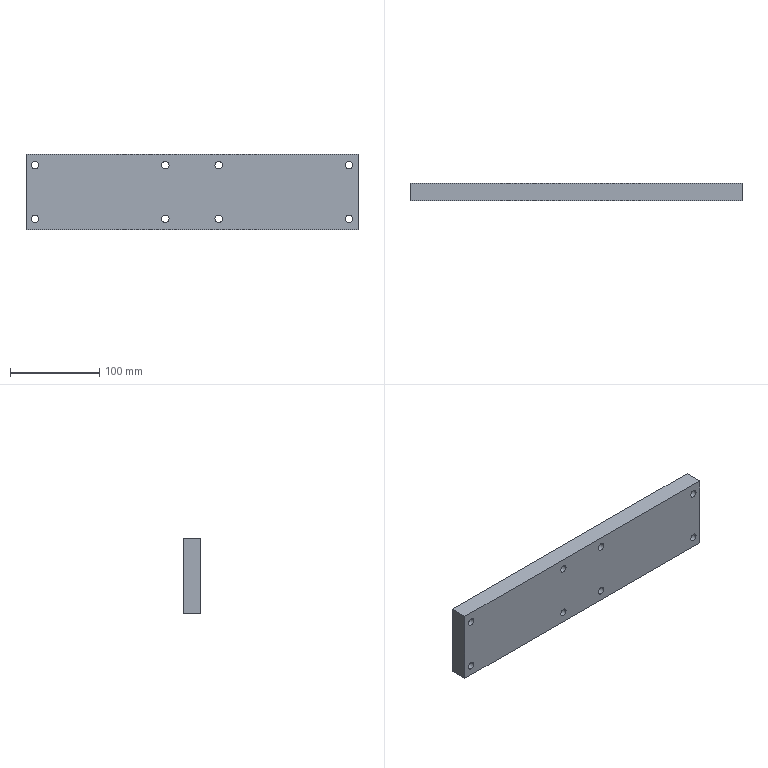Part | NX | features BREP 1 | 1 solid | 46 faces | box 372 x 20 x 85 mm | volume 616323 mm3 | cylinder 32 | plane 14 | commonest cylinder face diameters 8.5 x16 14 x16
STEP:
#1=CARTESIAN_POINT('',(-186.,0.,-42.5));
#2=VERTEX_POINT('',#1);
#3=CARTESIAN_POINT('',(-186.,0.,42.5));
#4=VERTEX_POINT('',#3);
#5=CARTESIAN_POINT('',(-186.,0.,-42.5));
#6=DIRECTION('',(0.,0.,1.));
#7=VECTOR('',#6,1000.);
#8=LINE('',#5,#7);
#9=EDGE_CURVE('',#2,#4,#8,.T.);
#10=ORIENTED_EDGE('',*,*,#9,.F.);
#11=CARTESIAN_POINT('',(186.,0.,-42.5));
#12=VERTEX_POINT('',#11);
#13=CARTESIAN_POINT('',(186.,0.,-42.5));
#14=DIRECTION('',(-1.,0.,0.));
#15=VECTOR('',#14,1000.);
#16=LINE('',#13,#15);
#17=EDGE_CURVE('',#12,#2,#16,.T.);
#18=ORIENTED_EDGE('',*,*,#17,.F.);
#19=CARTESIAN_POINT('',(186.,0.,42.5));
#20=VERTEX_POINT('',#19);
#21=CARTESIAN_POINT('',(186.,0.,42.5));
#22=DIRECTION('',(0.,0.,-1.));
#23=VECTOR('',#22,1000.);
#24=LINE('',#21,#23);
#25=EDGE_CURVE('',#20,#12,#24,.T.);
#26=ORIENTED_EDGE('',*,*,#25,.F.);
#27=CARTESIAN_POINT('',(-186.,0.,42.5));
#28=DIRECTION('',(1.,0.,0.));
#29=VECTOR('',#28,1000.);
#30=LINE('',#27,#29);
#31=EDGE_CURVE('',#4,#20,#30,.T.);
#32=ORIENTED_EDGE('',*,*,#31,.F.);
#33=EDGE_LOOP('',(#10,#18,#26,#32));
#34=FACE_BOUND('',#33,.T.);
#35=CARTESIAN_POINT('',(-34.25,0.,-30.));
#36=VERTEX_POINT('',#35);
#37=CARTESIAN_POINT('',(-25.75,0.,-30.));
#38=VERTEX_POINT('',#37);
#39=CARTESIAN_POINT('',(-30.,0.,-30.));
#40=DIRECTION('',(0.,1.,0.));
#41=DIRECTION('',(-1.,0.,0.));
#42=AXIS2_PLACEMENT_3D('',#39,#40,#41);
#43=CIRCLE('',#42,4.25);
#44=EDGE_CURVE('',#36,#38,#43,.T.);
#45=ORIENTED_EDGE('',*,*,#44,.T.);
#46=CARTESIAN_POINT('',(-30.,0.,-30.));
#47=DIRECTION('',(0.,1.,0.));
#48=DIRECTION('',(1.,0.,0.));
#49=AXIS2_PLACEMENT_3D('',#46,#47,#48);
#50=CIRCLE('',#49,4.25);
#51=EDGE_CURVE('',#38,#36,#50,.T.);
#52=ORIENTED_EDGE('',*,*,#51,.T.);
#53=EDGE_LOOP('',(#45,#52));
#54=FACE_BOUND('',#53,.T.);
#55=CARTESIAN_POINT('',(25.75,0.,-30.));
#56=VERTEX_POINT('',#55);
#57=CARTESIAN_POINT('',(34.25,0.,-30.));
#58=VERTEX_POINT('',#57);
#59=CARTESIAN_POINT('',(30.,0.,-30.));
#60=DIRECTION('',(0.,1.,0.));
#61=DIRECTION('',(-1.,0.,0.));
#62=AXIS2_PLACEMENT_3D('',#59,#60,#61);
#63=CIRCLE('',#62,4.25);
#64=EDGE_CURVE('',#56,#58,#63,.T.);
#65=ORIENTED_EDGE('',*,*,#64,.T.);
#66=CARTESIAN_POINT('',(30.,0.,-30.));
#67=DIRECTION('',(0.,1.,0.));
#68=DIRECTION('',(1.,0.,0.));
#69=AXIS2_PLACEMENT_3D('',#66,#67,#68);
#70=CIRCLE('',#69,4.25);
#71=EDGE_CURVE('',#58,#56,#70,.T.);
#72=ORIENTED_EDGE('',*,*,#71,.T.);
#73=EDGE_LOOP('',(#65,#72));
#74=FACE_BOUND('',#73,.T.);
#75=CARTESIAN_POINT('',(-34.25,0.,30.));
#76=VERTEX_POINT('',#75);
#77=CARTESIAN_POINT('',(-25.75,0.,30.));
#78=VERTEX_POINT('',#77);
#79=CARTESIAN_POINT('',(-30.,0.,30.));
#80=DIRECTION('',(0.,1.,0.));
#81=DIRECTION('',(-1.,0.,0.));
#82=AXIS2_PLACEMENT_3D('',#79,#80,#81);
#83=CIRCLE('',#82,4.25);
#84=EDGE_CURVE('',#76,#78,#83,.T.);
#85=ORIENTED_EDGE('',*,*,#84,.T.);
#86=CARTESIAN_POINT('',(-30.,0.,30.));
#87=DIRECTION('',(0.,1.,0.));
#88=DIRECTION('',(1.,0.,0.));
#89=AXIS2_PLACEMENT_3D('',#86,#87,#88);
#90=CIRCLE('',#89,4.25);
#91=EDGE_CURVE('',#78,#76,#90,.T.);
#92=ORIENTED_EDGE('',*,*,#91,.T.);
#93=EDGE_LOOP('',(#85,#92));
#94=FACE_BOUND('',#93,.T.);
#95=CARTESIAN_POINT('',(25.75,0.,30.));
#96=VERTEX_POINT('',#95);
#97=CARTESIAN_POINT('',(34.25,0.,30.));
#98=VERTEX_POINT('',#97);
#99=CARTESIAN_POINT('',(30.,0.,30.));
#100=DIRECTION('',(0.,1.,0.));
#101=DIRECTION('',(-1.,0.,0.));
#102=AXIS2_PLACEMENT_3D('',#99,#100,#101);
#103=CIRCLE('',#102,4.25);
#104=EDGE_CURVE('',#96,#98,#103,.T.);
#105=ORIENTED_EDGE('',*,*,#104,.T.);
#106=CARTESIAN_POINT('',(30.,0.,30.));
#107=DIRECTION('',(0.,1.,0.));
#108=DIRECTION('',(1.,0.,0.));
#109=AXIS2_PLACEMENT_3D('',#106,#107,#108);
#110=CIRCLE('',#109,4.25);
#111=EDGE_CURVE('',#98,#96,#110,.T.);
#112=ORIENTED_EDGE('',*,*,#111,.T.);
#113=EDGE_LOOP('',(#105,#112));
#114=FACE_BOUND('',#113,.T.);
#115=CARTESIAN_POINT('',(-180.25,0.,-30.));
#116=VERTEX_POINT('',#115);
#117=CARTESIAN_POINT('',(-171.75,0.,-30.));
#118=VERTEX_POINT('',#117);
#119=CARTESIAN_POINT('',(-176.,0.,-30.));
#120=DIRECTION('',(0.,1.,0.));
#121=DIRECTION('',(-1.,0.,0.));
#122=AXIS2_PLACEMENT_3D('',#119,#120,#121);
#123=CIRCLE('',#122,4.25);
#124=EDGE_CURVE('',#116,#118,#123,.T.);
#125=ORIENTED_EDGE('',*,*,#124,.T.);
#126=CARTESIAN_POINT('',(-176.,0.,-30.));
#127=DIRECTION('',(0.,1.,0.));
#128=DIRECTION('',(1.,0.,0.));
#129=AXIS2_PLACEMENT_3D('',#126,#127,#128);
#130=CIRCLE('',#129,4.25);
#131=EDGE_CURVE('',#118,#116,#130,.T.);
#132=ORIENTED_EDGE('',*,*,#131,.T.);
#133=EDGE_LOOP('',(#125,#132));
#134=FACE_BOUND('',#133,.T.);
#135=CARTESIAN_POINT('',(-180.25,0.,30.));
#136=VERTEX_POINT('',#135);
#137=CARTESIAN_POINT('',(-171.75,0.,30.));
#138=VERTEX_POINT('',#137);
#139=CARTESIAN_POINT('',(-176.,0.,30.));
#140=DIRECTION('',(0.,1.,0.));
#141=DIRECTION('',(-1.,0.,0.));
#142=AXIS2_PLACEMENT_3D('',#139,#140,#141);
#143=CIRCLE('',#142,4.25);
#144=EDGE_CURVE('',#136,#138,#143,.T.);
#145=ORIENTED_EDGE('',*,*,#144,.T.);
#146=CARTESIAN_POINT('',(-176.,0.,30.));
#147=DIRECTION('',(0.,1.,0.));
#148=DIRECTION('',(1.,0.,0.));
#149=AXIS2_PLACEMENT_3D('',#146,#147,#148);
#150=CIRCLE('',#149,4.25);
#151=EDGE_CURVE('',#138,#136,#150,.T.);
#152=ORIENTED_EDGE('',*,*,#151,.T.);
#153=EDGE_LOOP('',(#145,#152));
#154=FACE_BOUND('',#153,.T.);
#155=CARTESIAN_POINT('',(171.75,0.,-30.));
#156=VERTEX_POINT('',#155);
#157=CARTESIAN_POINT('',(180.25,0.,-30.));
#158=VERTEX_POINT('',#157);
#159=CARTESIAN_POINT('',(176.,0.,-30.));
#160=DIRECTION('',(0.,1.,0.));
#161=DIRECTION('',(-1.,0.,0.));
#162=AXIS2_PLACEMENT_3D('',#159,#160,#161);
#163=CIRCLE('',#162,4.25);
#164=EDGE_CURVE('',#156,#158,#163,.T.);
#165=ORIENTED_EDGE('',*,*,#164,.T.);
#166=CARTESIAN_POINT('',(176.,0.,-30.));
#167=DIRECTION('',(0.,1.,0.));
#168=DIRECTION('',(1.,0.,0.));
#169=AXIS2_PLACEMENT_3D('',#166,#167,#168);
#170=CIRCLE('',#169,4.25);
#171=EDGE_CURVE('',#158,#156,#170,.T.);
#172=ORIENTED_EDGE('',*,*,#171,.T.);
#173=EDGE_LOOP('',(#165,#172));
#174=FACE_BOUND('',#173,.T.);
#175=CARTESIAN_POINT('',(171.75,0.,30.));
#176=VERTEX_POINT('',#175);
#177=CARTESIAN_POINT('',(180.25,0.,30.));
#178=VERTEX_POINT('',#177);
#179=CARTESIAN_POINT('',(176.,0.,30.));
#180=DIRECTION('',(0.,1.,0.));
#181=DIRECTION('',(-1.,0.,0.));
#182=AXIS2_PLACEMENT_3D('',#179,#180,#181);
#183=CIRCLE('',#182,4.25);
#184=EDGE_CURVE('',#176,#178,#183,.T.);
#185=ORIENTED_EDGE('',*,*,#184,.T.);
#186=CARTESIAN_POINT('',(176.,0.,30.));
#187=DIRECTION('',(0.,1.,0.));
#188=DIRECTION('',(1.,0.,0.));
#189=AXIS2_PLACEMENT_3D('',#186,#187,#188);
#190=CIRCLE('',#189,4.25);
#191=EDGE_CURVE('',#178,#176,#190,.T.);
#192=ORIENTED_EDGE('',*,*,#191,.T.);
#193=EDGE_LOOP('',(#185,#192));
#194=FACE_BOUND('',#193,.T.);
#195=CARTESIAN_POINT('',(0.,0.,0.));
#196=DIRECTION('',(0.,1.,0.));
#197=DIRECTION('',(1.,0.,0.));
#198=AXIS2_PLACEMENT_3D('',#195,#196,#197);
#199=PLANE('',#198);
#200=ADVANCED_FACE('',(#34,#54,#74,#94,#114,#134,#154,#174,#194),#199,.F.);
#201=CARTESIAN_POINT('',(186.,20.,42.5));
#202=VERTEX_POINT('',#201);
#203=CARTESIAN_POINT('',(186.,0.,42.5));
#204=DIRECTION('',(0.,1.,0.));
#205=VECTOR('',#204,1000.);
#206=LINE('',#203,#205);
#207=EDGE_CURVE('',#20,#202,#206,.T.);
#208=ORIENTED_EDGE('',*,*,#207,.T.);
#209=CARTESIAN_POINT('',(-186.,20.,42.5));
#210=VERTEX_POINT('',#209);
#211=CARTESIAN_POINT('',(-186.,20.,42.5));
#212=DIRECTION('',(1.,0.,0.));
#213=VECTOR('',#212,1000.);
#214=LINE('',#211,#213);
#215=EDGE_CURVE('',#210,#202,#214,.T.);
#216=ORIENTED_EDGE('',*,*,#215,.F.);
#217=CARTESIAN_POINT('',(-186.,0.,42.5));
#218=DIRECTION('',(0.,1.,0.));
#219=VECTOR('',#218,1000.);
#220=LINE('',#217,#219);
#221=EDGE_CURVE('',#4,#210,#220,.T.);
#222=ORIENTED_EDGE('',*,*,#221,.F.);
#223=ORIENTED_EDGE('',*,*,#31,.T.);
#224=EDGE_LOOP('',(#208,#216,#222,#223));
#225=FACE_BOUND('',#224,.T.);
#226=CARTESIAN_POINT('',(-186.,0.,42.5));
#227=DIRECTION('',(0.,0.,1.));
#228=DIRECTION('',(1.,0.,0.));
#229=AXIS2_PLACEMENT_3D('',#226,#227,#228);
#230=PLANE('',#229);
#231=ADVANCED_FACE('',(#225),#230,.T.);
#232=ORIENTED_EDGE('',*,*,#221,.T.);
#233=CARTESIAN_POINT('',(-186.,20.,-42.5));
#234=VERTEX_POINT('',#233);
#235=CARTESIAN_POINT('',(-186.,20.,-42.5));
#236=DIRECTION('',(0.,0.,1.));
#237=VECTOR('',#236,1000.);
#238=LINE('',#235,#237);
#239=EDGE_CURVE('',#234,#210,#238,.T.);
#240=ORIENTED_EDGE('',*,*,#239,.F.);
#241=CARTESIAN_POINT('',(-186.,0.,-42.5));
#242=DIRECTION('',(0.,1.,0.));
#243=VECTOR('',#242,1000.);
#244=LINE('',#241,#243);
#245=EDGE_CURVE('',#2,#234,#244,.T.);
#246=ORIENTED_EDGE('',*,*,#245,.F.);
#247=ORIENTED_EDGE('',*,*,#9,.T.);
#248=EDGE_LOOP('',(#232,#240,#246,#247));
#249=FACE_BOUND('',#248,.T.);
#250=CARTESIAN_POINT('',(-186.,0.,-42.5));
#251=DIRECTION('',(-1.,0.,0.));
#252=DIRECTION('',(0.,0.,1.));
#253=AXIS2_PLACEMENT_3D('',#250,#251,#252);
#254=PLANE('',#253);
#255=ADVANCED_FACE('',(#249),#254,.T.);
#256=ORIENTED_EDGE('',*,*,#245,.T.);
#257=CARTESIAN_POINT('',(186.,20.,-42.5));
#258=VERTEX_POINT('',#257);
#259=CARTESIAN_POINT('',(186.,20.,-42.5));
#260=DIRECTION('',(-1.,0.,0.));
#261=VECTOR('',#260,1000.);
#262=LINE('',#259,#261);
#263=EDGE_CURVE('',#258,#234,#262,.T.);
#264=ORIENTED_EDGE('',*,*,#263,.F.);
#265=CARTESIAN_POINT('',(186.,0.,-42.5));
#266=DIRECTION('',(0.,1.,0.));
#267=VECTOR('',#266,1000.);
#268=LINE('',#265,#267);
#269=EDGE_CURVE('',#12,#258,#268,.T.);
#270=ORIENTED_EDGE('',*,*,#269,.F.);
#271=ORIENTED_EDGE('',*,*,#17,.T.);
#272=EDGE_LOOP('',(#256,#264,#270,#271));
#273=FACE_BOUND('',#272,.T.);
#274=CARTESIAN_POINT('',(186.,0.,-42.5));
#275=DIRECTION('',(0.,0.,-1.));
#276=DIRECTION('',(0.,-1.,0.));
#277=AXIS2_PLACEMENT_3D('',#274,#275,#276);
#278=PLANE('',#277);
#279=ADVANCED_FACE('',(#273),#278,.T.);
#280=ORIENTED_EDGE('',*,*,#269,.T.);
#281=CARTESIAN_POINT('',(186.,20.,42.5));
#282=DIRECTION('',(0.,0.,-1.));
#283=VECTOR('',#282,1000.);
#284=LINE('',#281,#283);
#285=EDGE_CURVE('',#202,#258,#284,.T.);
#286=ORIENTED_EDGE('',*,*,#285,.F.);
#287=ORIENTED_EDGE('',*,*,#207,.F.);
#288=ORIENTED_EDGE('',*,*,#25,.T.);
#289=EDGE_LOOP('',(#280,#286,#287,#288));
#290=FACE_BOUND('',#289,.T.);
#291=CARTESIAN_POINT('',(186.,0.,42.5));
#292=DIRECTION('',(1.,0.,0.));
#293=DIRECTION('',(0.,1.,0.));
#294=AXIS2_PLACEMENT_3D('',#291,#292,#293);
#295=PLANE('',#294);
#296=ADVANCED_FACE('',(#290),#295,.T.);
#297=ORIENTED_EDGE('',*,*,#285,.T.);
#298=ORIENTED_EDGE('',*,*,#263,.T.);
#299=ORIENTED_EDGE('',*,*,#239,.T.);
#300=ORIENTED_EDGE('',*,*,#215,.T.);
#301=EDGE_LOOP('',(#297,#298,#299,#300));
#302=FACE_BOUND('',#301,.T.);
#303=CARTESIAN_POINT('',(-37.,20.,-30.));
#304=VERTEX_POINT('',#303);
#305=CARTESIAN_POINT('',(-23.,20.,-30.));
#306=VERTEX_POINT('',#305);
#307=CARTESIAN_POINT('',(-30.,20.,-30.));
#308=DIRECTION('',(0.,1.,0.));
#309=DIRECTION('',(-1.,0.,0.));
#310=AXIS2_PLACEMENT_3D('',#307,#308,#309);
#311=CIRCLE('',#310,7.);
#312=EDGE_CURVE('',#304,#306,#311,.T.);
#313=ORIENTED_EDGE('',*,*,#312,.F.);
#314=CARTESIAN_POINT('',(-30.,20.,-30.));
#315=DIRECTION('',(0.,1.,0.));
#316=DIRECTION('',(1.,0.,0.));
#317=AXIS2_PLACEMENT_3D('',#314,#315,#316);
#318=CIRCLE('',#317,7.);
#319=EDGE_CURVE('',#306,#304,#318,.T.);
#320=ORIENTED_EDGE('',*,*,#319,.F.);
#321=EDGE_LOOP('',(#313,#320));
#322=FACE_BOUND('',#321,.T.);
#323=CARTESIAN_POINT('',(23.,20.,-30.));
#324=VERTEX_POINT('',#323);
#325=CARTESIAN_POINT('',(37.,20.,-30.));
#326=VERTEX_POINT('',#325);
#327=CARTESIAN_POINT('',(30.,20.,-30.));
#328=DIRECTION('',(0.,1.,0.));
#329=DIRECTION('',(-1.,0.,0.));
#330=AXIS2_PLACEMENT_3D('',#327,#328,#329);
#331=CIRCLE('',#330,7.);
#332=EDGE_CURVE('',#324,#326,#331,.T.);
#333=ORIENTED_EDGE('',*,*,#332,.F.);
#334=CARTESIAN_POINT('',(30.,20.,-30.));
#335=DIRECTION('',(0.,1.,0.));
#336=DIRECTION('',(1.,0.,0.));
#337=AXIS2_PLACEMENT_3D('',#334,#335,#336);
#338=CIRCLE('',#337,7.);
#339=EDGE_CURVE('',#326,#324,#338,.T.);
#340=ORIENTED_EDGE('',*,*,#339,.F.);
#341=EDGE_LOOP('',(#333,#340));
#342=FACE_BOUND('',#341,.T.);
#343=CARTESIAN_POINT('',(-37.,20.,30.));
#344=VERTEX_POINT('',#343);
#345=CARTESIAN_POINT('',(-23.,20.,30.));
#346=VERTEX_POINT('',#345);
#347=CARTESIAN_POINT('',(-30.,20.,30.));
#348=DIRECTION('',(0.,1.,0.));
#349=DIRECTION('',(-1.,0.,0.));
#350=AXIS2_PLACEMENT_3D('',#347,#348,#349);
#351=CIRCLE('',#350,7.);
#352=EDGE_CURVE('',#344,#346,#351,.T.);
#353=ORIENTED_EDGE('',*,*,#352,.F.);
#354=CARTESIAN_POINT('',(-30.,20.,30.));
#355=DIRECTION('',(0.,1.,0.));
#356=DIRECTION('',(1.,0.,0.));
#357=AXIS2_PLACEMENT_3D('',#354,#355,#356);
#358=CIRCLE('',#357,7.);
#359=EDGE_CURVE('',#346,#344,#358,.T.);
#360=ORIENTED_EDGE('',*,*,#359,.F.);
#361=EDGE_LOOP('',(#353,#360));
#362=FACE_BOUND('',#361,.T.);
#363=CARTESIAN_POINT('',(23.,20.,30.));
#364=VERTEX_POINT('',#363);
#365=CARTESIAN_POINT('',(37.,20.,30.));
#366=VERTEX_POINT('',#365);
#367=CARTESIAN_POINT('',(30.,20.,30.));
#368=DIRECTION('',(0.,1.,0.));
#369=DIRECTION('',(-1.,0.,0.));
#370=AXIS2_PLACEMENT_3D('',#367,#368,#369);
#371=CIRCLE('',#370,7.);
#372=EDGE_CURVE('',#364,#366,#371,.T.);
#373=ORIENTED_EDGE('',*,*,#372,.F.);
#374=CARTESIAN_POINT('',(30.,20.,30.));
#375=DIRECTION('',(0.,1.,0.));
#376=DIRECTION('',(1.,0.,0.));
#377=AXIS2_PLACEMENT_3D('',#374,#375,#376);
#378=CIRCLE('',#377,7.);
#379=EDGE_CURVE('',#366,#364,#378,.T.);
#380=ORIENTED_EDGE('',*,*,#379,.F.);
#381=EDGE_LOOP('',(#373,#380));
#382=FACE_BOUND('',#381,.T.);
#383=CARTESIAN_POINT('',(-183.,20.,-30.));
#384=VERTEX_POINT('',#383);
#385=CARTESIAN_POINT('',(-169.,20.,-30.));
#386=VERTEX_POINT('',#385);
#387=CARTESIAN_POINT('',(-176.,20.,-30.));
#388=DIRECTION('',(0.,1.,0.));
#389=DIRECTION('',(-1.,0.,0.));
#390=AXIS2_PLACEMENT_3D('',#387,#388,#389);
#391=CIRCLE('',#390,7.);
#392=EDGE_CURVE('',#384,#386,#391,.T.);
#393=ORIENTED_EDGE('',*,*,#392,.F.);
#394=CARTESIAN_POINT('',(-176.,20.,-30.));
#395=DIRECTION('',(0.,1.,0.));
#396=DIRECTION('',(1.,0.,0.));
#397=AXIS2_PLACEMENT_3D('',#394,#395,#396);
#398=CIRCLE('',#397,7.);
#399=EDGE_CURVE('',#386,#384,#398,.T.);
#400=ORIENTED_EDGE('',*,*,#399,.F.);
#401=EDGE_LOOP('',(#393,#400));
#402=FACE_BOUND('',#401,.T.);
#403=CARTESIAN_POINT('',(-183.,20.,30.));
#404=VERTEX_POINT('',#403);
#405=CARTESIAN_POINT('',(-169.,20.,30.));
#406=VERTEX_POINT('',#405);
#407=CARTESIAN_POINT('',(-176.,20.,30.));
#408=DIRECTION('',(0.,1.,0.));
#409=DIRECTION('',(-1.,0.,0.));
#410=AXIS2_PLACEMENT_3D('',#407,#408,#409);
#411=CIRCLE('',#410,7.);
#412=EDGE_CURVE('',#404,#406,#411,.T.);
#413=ORIENTED_EDGE('',*,*,#412,.F.);
#414=CARTESIAN_POINT('',(-176.,20.,30.));
#415=DIRECTION('',(0.,1.,0.));
#416=DIRECTION('',(1.,0.,0.));
#417=AXIS2_PLACEMENT_3D('',#414,#415,#416);
#418=CIRCLE('',#417,7.);
#419=EDGE_CURVE('',#406,#404,#418,.T.);
#420=ORIENTED_EDGE('',*,*,#419,.F.);
#421=EDGE_LOOP('',(#413,#420));
#422=FACE_BOUND('',#421,.T.);
#423=CARTESIAN_POINT('',(169.,20.,-30.));
#424=VERTEX_POINT('',#423);
#425=CARTESIAN_POINT('',(183.,20.,-30.));
#426=VERTEX_POINT('',#425);
#427=CARTESIAN_POINT('',(176.,20.,-30.));
#428=DIRECTION('',(0.,1.,0.));
#429=DIRECTION('',(-1.,0.,0.));
#430=AXIS2_PLACEMENT_3D('',#427,#428,#429);
#431=CIRCLE('',#430,7.);
#432=EDGE_CURVE('',#424,#426,#431,.T.);
#433=ORIENTED_EDGE('',*,*,#432,.F.);
#434=CARTESIAN_POINT('',(176.,20.,-30.));
#435=DIRECTION('',(0.,1.,0.));
#436=DIRECTION('',(1.,0.,0.));
#437=AXIS2_PLACEMENT_3D('',#434,#435,#436);
#438=CIRCLE('',#437,7.);
#439=EDGE_CURVE('',#426,#424,#438,.T.);
#440=ORIENTED_EDGE('',*,*,#439,.F.);
#441=EDGE_LOOP('',(#433,#440));
#442=FACE_BOUND('',#441,.T.);
#443=CARTESIAN_POINT('',(169.,20.,30.));
#444=VERTEX_POINT('',#443);
#445=CARTESIAN_POINT('',(183.,20.,30.));
#446=VERTEX_POINT('',#445);
#447=CARTESIAN_POINT('',(176.,20.,30.));
#448=DIRECTION('',(0.,1.,0.));
#449=DIRECTION('',(-1.,0.,0.));
#450=AXIS2_PLACEMENT_3D('',#447,#448,#449);
#451=CIRCLE('',#450,7.);
#452=EDGE_CURVE('',#444,#446,#451,.T.);
#453=ORIENTED_EDGE('',*,*,#452,.F.);
#454=CARTESIAN_POINT('',(176.,20.,30.));
#455=DIRECTION('',(0.,1.,0.));
#456=DIRECTION('',(1.,0.,0.));
#457=AXIS2_PLACEMENT_3D('',#454,#455,#456);
#458=CIRCLE('',#457,7.);
#459=EDGE_CURVE('',#446,#444,#458,.T.);
#460=ORIENTED_EDGE('',*,*,#459,.F.);
#461=EDGE_LOOP('',(#453,#460));
#462=FACE_BOUND('',#461,.T.);
#463=CARTESIAN_POINT('',(0.,20.,0.));
#464=DIRECTION('',(0.,1.,0.));
#465=DIRECTION('',(1.,0.,0.));
#466=AXIS2_PLACEMENT_3D('',#463,#464,#465);
#467=PLANE('',#466);
#468=ADVANCED_FACE('',(#302,#322,#342,#362,#382,#402,#422,#442,#462),#467,.T.);
#469=CARTESIAN_POINT('',(-37.,11.,-30.));
#470=VERTEX_POINT('',#469);
#471=CARTESIAN_POINT('',(-37.,11.,-30.));
#472=DIRECTION('',(0.,1.,0.));
#473=VECTOR('',#472,1000.);
#474=LINE('',#471,#473);
#475=EDGE_CURVE('',#470,#304,#474,.T.);
#476=ORIENTED_EDGE('',*,*,#475,.F.);
#477=CARTESIAN_POINT('',(-23.,11.,-30.));
#478=VERTEX_POINT('',#477);
#479=CARTESIAN_POINT('',(-30.,11.,-30.));
#480=DIRECTION('',(0.,1.,0.));
#481=DIRECTION('',(1.,0.,0.));
#482=AXIS2_PLACEMENT_3D('',#479,#480,#481);
#483=CIRCLE('',#482,7.);
#484=EDGE_CURVE('',#478,#470,#483,.T.);
#485=ORIENTED_EDGE('',*,*,#484,.F.);
#486=CARTESIAN_POINT('',(-23.,11.,-30.));
#487=DIRECTION('',(0.,1.,0.));
#488=VECTOR('',#487,1000.);
#489=LINE('',#486,#488);
#490=EDGE_CURVE('',#478,#306,#489,.T.);
#491=ORIENTED_EDGE('',*,*,#490,.T.);
#492=ORIENTED_EDGE('',*,*,#319,.T.);
#493=EDGE_LOOP('',(#476,#485,#491,#492));
#494=FACE_BOUND('',#493,.T.);
#495=CARTESIAN_POINT('',(-30.,-73.622,-30.));
#496=DIRECTION('',(0.,1.,0.));
#497=DIRECTION('',(1.,0.,0.));
#498=AXIS2_PLACEMENT_3D('',#495,#496,#497);
#499=CYLINDRICAL_SURFACE('',#498,7.);
#500=ADVANCED_FACE('',(#494),#499,.F.);
#501=ORIENTED_EDGE('',*,*,#490,.F.);
#502=CARTESIAN_POINT('',(-30.,11.,-30.));
#503=DIRECTION('',(0.,-1.,0.));
#504=DIRECTION('',(1.,0.,0.));
#505=AXIS2_PLACEMENT_3D('',#502,#503,#504);
#506=CIRCLE('',#505,7.);
#507=EDGE_CURVE('',#478,#470,#506,.T.);
#508=ORIENTED_EDGE('',*,*,#507,.T.);
#509=ORIENTED_EDGE('',*,*,#475,.T.);
#510=ORIENTED_EDGE('',*,*,#312,.T.);
#511=EDGE_LOOP('',(#501,#508,#509,#510));
#512=FACE_BOUND('',#511,.T.);
#513=CARTESIAN_POINT('',(-30.,-73.622,-30.));
#514=DIRECTION('',(0.,1.,0.));
#515=DIRECTION('',(1.,0.,0.));
#516=AXIS2_PLACEMENT_3D('',#513,#514,#515);
#517=CYLINDRICAL_SURFACE('',#516,7.);
#518=ADVANCED_FACE('',(#512),#517,.F.);
#519=ORIENTED_EDGE('',*,*,#507,.F.);
#520=ORIENTED_EDGE('',*,*,#484,.T.);
#521=EDGE_LOOP('',(#519,#520));
#522=FACE_BOUND('',#521,.T.);
#523=CARTESIAN_POINT('',(-25.75,11.,-30.));
#524=VERTEX_POINT('',#523);
#525=CARTESIAN_POINT('',(-34.25,11.,-30.));
#526=VERTEX_POINT('',#525);
#527=CARTESIAN_POINT('',(-30.,11.,-30.));
#528=DIRECTION('',(0.,1.,0.));
#529=DIRECTION('',(1.,0.,0.));
#530=AXIS2_PLACEMENT_3D('',#527,#528,#529);
#531=CIRCLE('',#530,4.25);
#532=EDGE_CURVE('',#524,#526,#531,.T.);
#533=ORIENTED_EDGE('',*,*,#532,.F.);
#534=CARTESIAN_POINT('',(-30.,11.,-30.));
#535=DIRECTION('',(0.,-1.,0.));
#536=DIRECTION('',(1.,0.,0.));
#537=AXIS2_PLACEMENT_3D('',#534,#535,#536);
#538=CIRCLE('',#537,4.25);
#539=EDGE_CURVE('',#524,#526,#538,.T.);
#540=ORIENTED_EDGE('',*,*,#539,.T.);
#541=EDGE_LOOP('',(#533,#540));
#542=FACE_BOUND('',#541,.T.);
#543=CARTESIAN_POINT('',(-30.,11.,-30.));
#544=DIRECTION('',(0.,1.,0.));
#545=DIRECTION('',(1.,0.,0.));
#546=AXIS2_PLACEMENT_3D('',#543,#544,#545);
#547=PLANE('',#546);
#548=ADVANCED_FACE('',(#522,#542),#547,.T.);
#549=ORIENTED_EDGE('',*,*,#44,.F.);
#550=CARTESIAN_POINT('',(-34.25,0.,-30.));
#551=DIRECTION('',(0.,1.,0.));
#552=VECTOR('',#551,1000.);
#553=LINE('',#550,#552);
#554=EDGE_CURVE('',#526,#36,#553,.F.);
#555=ORIENTED_EDGE('',*,*,#554,.F.);
#556=ORIENTED_EDGE('',*,*,#539,.F.);
#557=CARTESIAN_POINT('',(-25.75,0.,-30.));
#558=DIRECTION('',(0.,1.,0.));
#559=VECTOR('',#558,1000.);
#560=LINE('',#557,#559);
#561=EDGE_CURVE('',#524,#38,#560,.F.);
#562=ORIENTED_EDGE('',*,*,#561,.T.);
#563=EDGE_LOOP('',(#549,#555,#556,#562));
#564=FACE_BOUND('',#563,.T.);
#565=CARTESIAN_POINT('',(-30.,-73.622,-30.));
#566=DIRECTION('',(0.,1.,0.));
#567=DIRECTION('',(1.,0.,0.));
#568=AXIS2_PLACEMENT_3D('',#565,#566,#567);
#569=CYLINDRICAL_SURFACE('',#568,4.25);
#570=ADVANCED_FACE('',(#564),#569,.F.);
#571=ORIENTED_EDGE('',*,*,#532,.T.);
#572=ORIENTED_EDGE('',*,*,#554,.T.);
#573=ORIENTED_EDGE('',*,*,#51,.F.);
#574=ORIENTED_EDGE('',*,*,#561,.F.);
#575=EDGE_LOOP('',(#571,#572,#573,#574));
#576=FACE_BOUND('',#575,.T.);
#577=CARTESIAN_POINT('',(-30.,-73.622,-30.));
#578=DIRECTION('',(0.,1.,0.));
#579=DIRECTION('',(1.,0.,0.));
#580=AXIS2_PLACEMENT_3D('',#577,#578,#579);
#581=CYLINDRICAL_SURFACE('',#580,4.25);
#582=ADVANCED_FACE('',(#576),#581,.F.);
#583=CARTESIAN_POINT('',(23.,11.,-30.));
#584=VERTEX_POINT('',#583);
#585=CARTESIAN_POINT('',(23.,11.,-30.));
#586=DIRECTION('',(0.,1.,0.));
#587=VECTOR('',#586,1000.);
#588=LINE('',#585,#587);
#589=EDGE_CURVE('',#584,#324,#588,.T.);
#590=ORIENTED_EDGE('',*,*,#589,.F.);
#591=CARTESIAN_POINT('',(37.,11.,-30.));
#592=VERTEX_POINT('',#591);
#593=CARTESIAN_POINT('',(30.,11.,-30.));
#594=DIRECTION('',(0.,1.,0.));
#595=DIRECTION('',(1.,0.,0.));
#596=AXIS2_PLACEMENT_3D('',#593,#594,#595);
#597=CIRCLE('',#596,7.);
#598=EDGE_CURVE('',#592,#584,#597,.T.);
#599=ORIENTED_EDGE('',*,*,#598,.F.);
#600=CARTESIAN_POINT('',(37.,11.,-30.));
#601=DIRECTION('',(0.,1.,0.));
#602=VECTOR('',#601,1000.);
#603=LINE('',#600,#602);
#604=EDGE_CURVE('',#592,#326,#603,.T.);
#605=ORIENTED_EDGE('',*,*,#604,.T.);
#606=ORIENTED_EDGE('',*,*,#339,.T.);
#607=EDGE_LOOP('',(#590,#599,#605,#606));
#608=FACE_BOUND('',#607,.T.);
#609=CARTESIAN_POINT('',(30.,-73.622,-30.));
#610=DIRECTION('',(0.,1.,0.));
#611=DIRECTION('',(1.,0.,0.));
#612=AXIS2_PLACEMENT_3D('',#609,#610,#611);
#613=CYLINDRICAL_SURFACE('',#612,7.);
#614=ADVANCED_FACE('',(#608),#613,.F.);
#615=ORIENTED_EDGE('',*,*,#604,.F.);
#616=CARTESIAN_POINT('',(30.,11.,-30.));
#617=DIRECTION('',(0.,-1.,0.));
#618=DIRECTION('',(1.,0.,0.));
#619=AXIS2_PLACEMENT_3D('',#616,#617,#618);
#620=CIRCLE('',#619,7.);
#621=EDGE_CURVE('',#592,#584,#620,.T.);
#622=ORIENTED_EDGE('',*,*,#621,.T.);
#623=ORIENTED_EDGE('',*,*,#589,.T.);
#624=ORIENTED_EDGE('',*,*,#332,.T.);
#625=EDGE_LOOP('',(#615,#622,#623,#624));
#626=FACE_BOUND('',#625,.T.);
#627=CARTESIAN_POINT('',(30.,-73.622,-30.));
#628=DIRECTION('',(0.,1.,0.));
#629=DIRECTION('',(1.,0.,0.));
#630=AXIS2_PLACEMENT_3D('',#627,#628,#629);
#631=CYLINDRICAL_SURFACE('',#630,7.);
#632=ADVANCED_FACE('',(#626),#631,.F.);
#633=ORIENTED_EDGE('',*,*,#621,.F.);
#634=ORIENTED_EDGE('',*,*,#598,.T.);
#635=EDGE_LOOP('',(#633,#634));
#636=FACE_BOUND('',#635,.T.);
#637=CARTESIAN_POINT('',(34.25,11.,-30.));
#638=VERTEX_POINT('',#637);
#639=CARTESIAN_POINT('',(25.75,11.,-30.));
#640=VERTEX_POINT('',#639);
#641=CARTESIAN_POINT('',(30.,11.,-30.));
#642=DIRECTION('',(0.,1.,0.));
#643=DIRECTION('',(1.,0.,0.));
#644=AXIS2_PLACEMENT_3D('',#641,#642,#643);
#645=CIRCLE('',#644,4.25);
#646=EDGE_CURVE('',#638,#640,#645,.T.);
#647=ORIENTED_EDGE('',*,*,#646,.F.);
#648=CARTESIAN_POINT('',(30.,11.,-30.));
#649=DIRECTION('',(0.,-1.,0.));
#650=DIRECTION('',(1.,0.,0.));
#651=AXIS2_PLACEMENT_3D('',#648,#649,#650);
#652=CIRCLE('',#651,4.25);
#653=EDGE_CURVE('',#638,#640,#652,.T.);
#654=ORIENTED_EDGE('',*,*,#653,.T.);
#655=EDGE_LOOP('',(#647,#654));
#656=FACE_BOUND('',#655,.T.);
#657=CARTESIAN_POINT('',(30.,11.,-30.));
#658=DIRECTION('',(0.,1.,0.));
#659=DIRECTION('',(1.,0.,0.));
#660=AXIS2_PLACEMENT_3D('',#657,#658,#659);
#661=PLANE('',#660);
#662=ADVANCED_FACE('',(#636,#656),#661,.T.);
#663=ORIENTED_EDGE('',*,*,#64,.F.);
#664=CARTESIAN_POINT('',(25.75,0.,-30.));
#665=DIRECTION('',(0.,1.,0.));
#666=VECTOR('',#665,1000.);
#667=LINE('',#664,#666);
#668=EDGE_CURVE('',#640,#56,#667,.F.);
#669=ORIENTED_EDGE('',*,*,#668,.F.);
#670=ORIENTED_EDGE('',*,*,#653,.F.);
#671=CARTESIAN_POINT('',(34.25,0.,-30.));
#672=DIRECTION('',(0.,1.,0.));
#673=VECTOR('',#672,1000.);
#674=LINE('',#671,#673);
#675=EDGE_CURVE('',#638,#58,#674,.F.);
#676=ORIENTED_EDGE('',*,*,#675,.T.);
#677=EDGE_LOOP('',(#663,#669,#670,#676));
#678=FACE_BOUND('',#677,.T.);
#679=CARTESIAN_POINT('',(30.,-73.622,-30.));
#680=DIRECTION('',(0.,1.,0.));
#681=DIRECTION('',(1.,0.,0.));
#682=AXIS2_PLACEMENT_3D('',#679,#680,#681);
#683=CYLINDRICAL_SURFACE('',#682,4.25);
#684=ADVANCED_FACE('',(#678),#683,.F.);
#685=ORIENTED_EDGE('',*,*,#646,.T.);
#686=ORIENTED_EDGE('',*,*,#668,.T.);
#687=ORIENTED_EDGE('',*,*,#71,.F.);
#688=ORIENTED_EDGE('',*,*,#675,.F.);
#689=EDGE_LOOP('',(#685,#686,#687,#688));
#690=FACE_BOUND('',#689,.T.);
#691=CARTESIAN_POINT('',(30.,-73.622,-30.));
#692=DIRECTION('',(0.,1.,0.));
#693=DIRECTION('',(1.,0.,0.));
#694=AXIS2_PLACEMENT_3D('',#691,#692,#693);
#695=CYLINDRICAL_SURFACE('',#694,4.25);
#696=ADVANCED_FACE('',(#690),#695,.F.);
#697=CARTESIAN_POINT('',(-37.,11.,30.));
#698=VERTEX_POINT('',#697);
#699=CARTESIAN_POINT('',(-37.,11.,30.));
#700=DIRECTION('',(0.,1.,0.));
#701=VECTOR('',#700,1000.);
#702=LINE('',#699,#701);
#703=EDGE_CURVE('',#698,#344,#702,.T.);
#704=ORIENTED_EDGE('',*,*,#703,.F.);
#705=CARTESIAN_POINT('',(-23.,11.,30.));
#706=VERTEX_POINT('',#705);
#707=CARTESIAN_POINT('',(-30.,11.,30.));
#708=DIRECTION('',(0.,1.,0.));
#709=DIRECTION('',(1.,0.,0.));
#710=AXIS2_PLACEMENT_3D('',#707,#708,#709);
#711=CIRCLE('',#710,7.);
#712=EDGE_CURVE('',#706,#698,#711,.T.);
#713=ORIENTED_EDGE('',*,*,#712,.F.);
#714=CARTESIAN_POINT('',(-23.,11.,30.));
#715=DIRECTION('',(0.,1.,0.));
#716=VECTOR('',#715,1000.);
#717=LINE('',#714,#716);
#718=EDGE_CURVE('',#706,#346,#717,.T.);
#719=ORIENTED_EDGE('',*,*,#718,.T.);
#720=ORIENTED_EDGE('',*,*,#359,.T.);
#721=EDGE_LOOP('',(#704,#713,#719,#720));
#722=FACE_BOUND('',#721,.T.);
#723=CARTESIAN_POINT('',(-30.,-73.622,30.));
#724=DIRECTION('',(0.,1.,0.));
#725=DIRECTION('',(1.,0.,0.));
#726=AXIS2_PLACEMENT_3D('',#723,#724,#725);
#727=CYLINDRICAL_SURFACE('',#726,7.);
#728=ADVANCED_FACE('',(#722),#727,.F.);
#729=ORIENTED_EDGE('',*,*,#718,.F.);
#730=CARTESIAN_POINT('',(-30.,11.,30.));
#731=DIRECTION('',(0.,-1.,0.));
#732=DIRECTION('',(1.,0.,0.));
#733=AXIS2_PLACEMENT_3D('',#730,#731,#732);
#734=CIRCLE('',#733,7.);
#735=EDGE_CURVE('',#706,#698,#734,.T.);
#736=ORIENTED_EDGE('',*,*,#735,.T.);
#737=ORIENTED_EDGE('',*,*,#703,.T.);
#738=ORIENTED_EDGE('',*,*,#352,.T.);
#739=EDGE_LOOP('',(#729,#736,#737,#738));
#740=FACE_BOUND('',#739,.T.);
#741=CARTESIAN_POINT('',(-30.,-73.622,30.));
#742=DIRECTION('',(0.,1.,0.));
#743=DIRECTION('',(1.,0.,0.));
#744=AXIS2_PLACEMENT_3D('',#741,#742,#743);
#745=CYLINDRICAL_SURFACE('',#744,7.);
#746=ADVANCED_FACE('',(#740),#745,.F.);
#747=ORIENTED_EDGE('',*,*,#735,.F.);
#748=ORIENTED_EDGE('',*,*,#712,.T.);
#749=EDGE_LOOP('',(#747,#748));
#750=FACE_BOUND('',#749,.T.);
#751=CARTESIAN_POINT('',(-25.75,11.,30.));
#752=VERTEX_POINT('',#751);
#753=CARTESIAN_POINT('',(-34.25,11.,30.));
#754=VERTEX_POINT('',#753);
#755=CARTESIAN_POINT('',(-30.,11.,30.));
#756=DIRECTION('',(0.,1.,0.));
#757=DIRECTION('',(1.,0.,0.));
#758=AXIS2_PLACEMENT_3D('',#755,#756,#757);
#759=CIRCLE('',#758,4.25);
#760=EDGE_CURVE('',#752,#754,#759,.T.);
#761=ORIENTED_EDGE('',*,*,#760,.F.);
#762=CARTESIAN_POINT('',(-30.,11.,30.));
#763=DIRECTION('',(0.,-1.,0.));
#764=DIRECTION('',(1.,0.,0.));
#765=AXIS2_PLACEMENT_3D('',#762,#763,#764);
#766=CIRCLE('',#765,4.25);
#767=EDGE_CURVE('',#752,#754,#766,.T.);
#768=ORIENTED_EDGE('',*,*,#767,.T.);
#769=EDGE_LOOP('',(#761,#768));
#770=FACE_BOUND('',#769,.T.);
#771=CARTESIAN_POINT('',(-30.,11.,30.));
#772=DIRECTION('',(0.,1.,0.));
#773=DIRECTION('',(1.,0.,0.));
#774=AXIS2_PLACEMENT_3D('',#771,#772,#773);
#775=PLANE('',#774);
#776=ADVANCED_FACE('',(#750,#770),#775,.T.);
#777=ORIENTED_EDGE('',*,*,#84,.F.);
#778=CARTESIAN_POINT('',(-34.25,0.,30.));
#779=DIRECTION('',(0.,1.,0.));
#780=VECTOR('',#779,1000.);
#781=LINE('',#778,#780);
#782=EDGE_CURVE('',#754,#76,#781,.F.);
#783=ORIENTED_EDGE('',*,*,#782,.F.);
#784=ORIENTED_EDGE('',*,*,#767,.F.);
#785=CARTESIAN_POINT('',(-25.75,0.,30.));
#786=DIRECTION('',(0.,1.,0.));
#787=VECTOR('',#786,1000.);
#788=LINE('',#785,#787);
#789=EDGE_CURVE('',#752,#78,#788,.F.);
#790=ORIENTED_EDGE('',*,*,#789,.T.);
#791=EDGE_LOOP('',(#777,#783,#784,#790));
#792=FACE_BOUND('',#791,.T.);
#793=CARTESIAN_POINT('',(-30.,-73.622,30.));
#794=DIRECTION('',(0.,1.,0.));
#795=DIRECTION('',(1.,0.,0.));
#796=AXIS2_PLACEMENT_3D('',#793,#794,#795);
#797=CYLINDRICAL_SURFACE('',#796,4.25);
#798=ADVANCED_FACE('',(#792),#797,.F.);
#799=ORIENTED_EDGE('',*,*,#760,.T.);
#800=ORIENTED_EDGE('',*,*,#782,.T.);
#801=ORIENTED_EDGE('',*,*,#91,.F.);
#802=ORIENTED_EDGE('',*,*,#789,.F.);
#803=EDGE_LOOP('',(#799,#800,#801,#802));
#804=FACE_BOUND('',#803,.T.);
#805=CARTESIAN_POINT('',(-30.,-73.622,30.));
#806=DIRECTION('',(0.,1.,0.));
#807=DIRECTION('',(1.,0.,0.));
#808=AXIS2_PLACEMENT_3D('',#805,#806,#807);
#809=CYLINDRICAL_SURFACE('',#808,4.25);
#810=ADVANCED_FACE('',(#804),#809,.F.);
#811=CARTESIAN_POINT('',(23.,11.,30.));
#812=VERTEX_POINT('',#811);
#813=CARTESIAN_POINT('',(23.,11.,30.));
#814=DIRECTION('',(0.,1.,0.));
#815=VECTOR('',#814,1000.);
#816=LINE('',#813,#815);
#817=EDGE_CURVE('',#812,#364,#816,.T.);
#818=ORIENTED_EDGE('',*,*,#817,.F.);
#819=CARTESIAN_POINT('',(37.,11.,30.));
#820=VERTEX_POINT('',#819);
#821=CARTESIAN_POINT('',(30.,11.,30.));
#822=DIRECTION('',(0.,1.,0.));
#823=DIRECTION('',(1.,0.,0.));
#824=AXIS2_PLACEMENT_3D('',#821,#822,#823);
#825=CIRCLE('',#824,7.);
#826=EDGE_CURVE('',#820,#812,#825,.T.);
#827=ORIENTED_EDGE('',*,*,#826,.F.);
#828=CARTESIAN_POINT('',(37.,11.,30.));
#829=DIRECTION('',(0.,1.,0.));
#830=VECTOR('',#829,1000.);
#831=LINE('',#828,#830);
#832=EDGE_CURVE('',#820,#366,#831,.T.);
#833=ORIENTED_EDGE('',*,*,#832,.T.);
#834=ORIENTED_EDGE('',*,*,#379,.T.);
#835=EDGE_LOOP('',(#818,#827,#833,#834));
#836=FACE_BOUND('',#835,.T.);
#837=CARTESIAN_POINT('',(30.,-73.622,30.));
#838=DIRECTION('',(0.,1.,0.));
#839=DIRECTION('',(1.,0.,0.));
#840=AXIS2_PLACEMENT_3D('',#837,#838,#839);
#841=CYLINDRICAL_SURFACE('',#840,7.);
#842=ADVANCED_FACE('',(#836),#841,.F.);
#843=ORIENTED_EDGE('',*,*,#832,.F.);
#844=CARTESIAN_POINT('',(30.,11.,30.));
#845=DIRECTION('',(0.,-1.,0.));
#846=DIRECTION('',(1.,0.,0.));
#847=AXIS2_PLACEMENT_3D('',#844,#845,#846);
#848=CIRCLE('',#847,7.);
#849=EDGE_CURVE('',#820,#812,#848,.T.);
#850=ORIENTED_EDGE('',*,*,#849,.T.);
#851=ORIENTED_EDGE('',*,*,#817,.T.);
#852=ORIENTED_EDGE('',*,*,#372,.T.);
#853=EDGE_LOOP('',(#843,#850,#851,#852));
#854=FACE_BOUND('',#853,.T.);
#855=CARTESIAN_POINT('',(30.,-73.622,30.));
#856=DIRECTION('',(0.,1.,0.));
#857=DIRECTION('',(1.,0.,0.));
#858=AXIS2_PLACEMENT_3D('',#855,#856,#857);
#859=CYLINDRICAL_SURFACE('',#858,7.);
#860=ADVANCED_FACE('',(#854),#859,.F.);
#861=ORIENTED_EDGE('',*,*,#849,.F.);
#862=ORIENTED_EDGE('',*,*,#826,.T.);
#863=EDGE_LOOP('',(#861,#862));
#864=FACE_BOUND('',#863,.T.);
#865=CARTESIAN_POINT('',(34.25,11.,30.));
#866=VERTEX_POINT('',#865);
#867=CARTESIAN_POINT('',(25.75,11.,30.));
#868=VERTEX_POINT('',#867);
#869=CARTESIAN_POINT('',(30.,11.,30.));
#870=DIRECTION('',(0.,1.,0.));
#871=DIRECTION('',(1.,0.,0.));
#872=AXIS2_PLACEMENT_3D('',#869,#870,#871);
#873=CIRCLE('',#872,4.25);
#874=EDGE_CURVE('',#866,#868,#873,.T.);
#875=ORIENTED_EDGE('',*,*,#874,.F.);
#876=CARTESIAN_POINT('',(30.,11.,30.));
#877=DIRECTION('',(0.,-1.,0.));
#878=DIRECTION('',(1.,0.,0.));
#879=AXIS2_PLACEMENT_3D('',#876,#877,#878);
#880=CIRCLE('',#879,4.25);
#881=EDGE_CURVE('',#866,#868,#880,.T.);
#882=ORIENTED_EDGE('',*,*,#881,.T.);
#883=EDGE_LOOP('',(#875,#882));
#884=FACE_BOUND('',#883,.T.);
#885=CARTESIAN_POINT('',(30.,11.,30.));
#886=DIRECTION('',(0.,1.,0.));
#887=DIRECTION('',(1.,0.,0.));
#888=AXIS2_PLACEMENT_3D('',#885,#886,#887);
#889=PLANE('',#888);
#890=ADVANCED_FACE('',(#864,#884),#889,.T.);
#891=ORIENTED_EDGE('',*,*,#104,.F.);
#892=CARTESIAN_POINT('',(25.75,0.,30.));
#893=DIRECTION('',(0.,1.,0.));
#894=VECTOR('',#893,1000.);
#895=LINE('',#892,#894);
#896=EDGE_CURVE('',#868,#96,#895,.F.);
#897=ORIENTED_EDGE('',*,*,#896,.F.);
#898=ORIENTED_EDGE('',*,*,#881,.F.);
#899=CARTESIAN_POINT('',(34.25,0.,30.));
#900=DIRECTION('',(0.,1.,0.));
#901=VECTOR('',#900,1000.);
#902=LINE('',#899,#901);
#903=EDGE_CURVE('',#866,#98,#902,.F.);
#904=ORIENTED_EDGE('',*,*,#903,.T.);
#905=EDGE_LOOP('',(#891,#897,#898,#904));
#906=FACE_BOUND('',#905,.T.);
#907=CARTESIAN_POINT('',(30.,-73.622,30.));
#908=DIRECTION('',(0.,1.,0.));
#909=DIRECTION('',(1.,0.,0.));
#910=AXIS2_PLACEMENT_3D('',#907,#908,#909);
#911=CYLINDRICAL_SURFACE('',#910,4.25);
#912=ADVANCED_FACE('',(#906),#911,.F.);
#913=ORIENTED_EDGE('',*,*,#874,.T.);
#914=ORIENTED_EDGE('',*,*,#896,.T.);
#915=ORIENTED_EDGE('',*,*,#111,.F.);
#916=ORIENTED_EDGE('',*,*,#903,.F.);
#917=EDGE_LOOP('',(#913,#914,#915,#916));
#918=FACE_BOUND('',#917,.T.);
#919=CARTESIAN_POINT('',(30.,-73.622,30.));
#920=DIRECTION('',(0.,1.,0.));
#921=DIRECTION('',(1.,0.,0.));
#922=AXIS2_PLACEMENT_3D('',#919,#920,#921);
#923=CYLINDRICAL_SURFACE('',#922,4.25);
#924=ADVANCED_FACE('',(#918),#923,.F.);
#925=CARTESIAN_POINT('',(-183.,11.,-30.));
#926=VERTEX_POINT('',#925);
#927=CARTESIAN_POINT('',(-183.,11.,-30.));
#928=DIRECTION('',(0.,1.,0.));
#929=VECTOR('',#928,1000.);
#930=LINE('',#927,#929);
#931=EDGE_CURVE('',#926,#384,#930,.T.);
#932=ORIENTED_EDGE('',*,*,#931,.F.);
#933=CARTESIAN_POINT('',(-169.,11.,-30.));
#934=VERTEX_POINT('',#933);
#935=CARTESIAN_POINT('',(-176.,11.,-30.));
#936=DIRECTION('',(0.,1.,0.));
#937=DIRECTION('',(1.,0.,0.));
#938=AXIS2_PLACEMENT_3D('',#935,#936,#937);
#939=CIRCLE('',#938,7.);
#940=EDGE_CURVE('',#934,#926,#939,.T.);
#941=ORIENTED_EDGE('',*,*,#940,.F.);
#942=CARTESIAN_POINT('',(-169.,11.,-30.));
#943=DIRECTION('',(0.,1.,0.));
#944=VECTOR('',#943,1000.);
#945=LINE('',#942,#944);
#946=EDGE_CURVE('',#934,#386,#945,.T.);
#947=ORIENTED_EDGE('',*,*,#946,.T.);
#948=ORIENTED_EDGE('',*,*,#399,.T.);
#949=EDGE_LOOP('',(#932,#941,#947,#948));
#950=FACE_BOUND('',#949,.T.);
#951=CARTESIAN_POINT('',(-176.,-73.622,-30.));
#952=DIRECTION('',(0.,1.,0.));
#953=DIRECTION('',(1.,0.,0.));
#954=AXIS2_PLACEMENT_3D('',#951,#952,#953);
#955=CYLINDRICAL_SURFACE('',#954,7.);
#956=ADVANCED_FACE('',(#950),#955,.F.);
#957=ORIENTED_EDGE('',*,*,#946,.F.);
#958=CARTESIAN_POINT('',(-176.,11.,-30.));
#959=DIRECTION('',(0.,-1.,0.));
#960=DIRECTION('',(1.,0.,0.));
#961=AXIS2_PLACEMENT_3D('',#958,#959,#960);
#962=CIRCLE('',#961,7.);
#963=EDGE_CURVE('',#934,#926,#962,.T.);
#964=ORIENTED_EDGE('',*,*,#963,.T.);
#965=ORIENTED_EDGE('',*,*,#931,.T.);
#966=ORIENTED_EDGE('',*,*,#392,.T.);
#967=EDGE_LOOP('',(#957,#964,#965,#966));
#968=FACE_BOUND('',#967,.T.);
#969=CARTESIAN_POINT('',(-176.,-73.622,-30.));
#970=DIRECTION('',(0.,1.,0.));
#971=DIRECTION('',(1.,0.,0.));
#972=AXIS2_PLACEMENT_3D('',#969,#970,#971);
#973=CYLINDRICAL_SURFACE('',#972,7.);
#974=ADVANCED_FACE('',(#968),#973,.F.);
#975=ORIENTED_EDGE('',*,*,#963,.F.);
#976=ORIENTED_EDGE('',*,*,#940,.T.);
#977=EDGE_LOOP('',(#975,#976));
#978=FACE_BOUND('',#977,.T.);
#979=CARTESIAN_POINT('',(-171.75,11.,-30.));
#980=VERTEX_POINT('',#979);
#981=CARTESIAN_POINT('',(-180.25,11.,-30.));
#982=VERTEX_POINT('',#981);
#983=CARTESIAN_POINT('',(-176.,11.,-30.));
#984=DIRECTION('',(0.,1.,0.));
#985=DIRECTION('',(1.,0.,0.));
#986=AXIS2_PLACEMENT_3D('',#983,#984,#985);
#987=CIRCLE('',#986,4.25);
#988=EDGE_CURVE('',#980,#982,#987,.T.);
#989=ORIENTED_EDGE('',*,*,#988,.F.);
#990=CARTESIAN_POINT('',(-176.,11.,-30.));
#991=DIRECTION('',(0.,-1.,0.));
#992=DIRECTION('',(1.,0.,0.));
#993=AXIS2_PLACEMENT_3D('',#990,#991,#992);
#994=CIRCLE('',#993,4.25);
#995=EDGE_CURVE('',#980,#982,#994,.T.);
#996=ORIENTED_EDGE('',*,*,#995,.T.);
#997=EDGE_LOOP('',(#989,#996));
#998=FACE_BOUND('',#997,.T.);
#999=CARTESIAN_POINT('',(-176.,11.,-30.));
#1000=DIRECTION('',(0.,1.,0.));
#1001=DIRECTION('',(1.,0.,0.));
#1002=AXIS2_PLACEMENT_3D('',#999,#1000,#1001);
#1003=PLANE('',#1002);
#1004=ADVANCED_FACE('',(#978,#998),#1003,.T.);
#1005=CARTESIAN_POINT('',(-180.25,0.,-30.));
#1006=DIRECTION('',(0.,1.,0.));
#1007=VECTOR('',#1006,1000.);
#1008=LINE('',#1005,#1007);
#1009=EDGE_CURVE('',#116,#982,#1008,.T.);
#1010=ORIENTED_EDGE('',*,*,#1009,.T.);
#1011=ORIENTED_EDGE('',*,*,#995,.F.);
#1012=CARTESIAN_POINT('',(-171.75,0.,-30.));
#1013=DIRECTION('',(0.,1.,0.));
#1014=VECTOR('',#1013,1000.);
#1015=LINE('',#1012,#1014);
#1016=EDGE_CURVE('',#118,#980,#1015,.T.);
#1017=ORIENTED_EDGE('',*,*,#1016,.F.);
#1018=ORIENTED_EDGE('',*,*,#124,.F.);
#1019=EDGE_LOOP('',(#1010,#1011,#1017,#1018));
#1020=FACE_BOUND('',#1019,.T.);
#1021=CARTESIAN_POINT('',(-176.,-73.622,-30.));
#1022=DIRECTION('',(0.,1.,0.));
#1023=DIRECTION('',(1.,0.,0.));
#1024=AXIS2_PLACEMENT_3D('',#1021,#1022,#1023);
#1025=CYLINDRICAL_SURFACE('',#1024,4.25);
#1026=ADVANCED_FACE('',(#1020),#1025,.F.);
#1027=ORIENTED_EDGE('',*,*,#1016,.T.);
#1028=ORIENTED_EDGE('',*,*,#988,.T.);
#1029=ORIENTED_EDGE('',*,*,#1009,.F.);
#1030=ORIENTED_EDGE('',*,*,#131,.F.);
#1031=EDGE_LOOP('',(#1027,#1028,#1029,#1030));
#1032=FACE_BOUND('',#1031,.T.);
#1033=CARTESIAN_POINT('',(-176.,-73.622,-30.));
#1034=DIRECTION('',(0.,1.,0.));
#1035=DIRECTION('',(1.,0.,0.));
#1036=AXIS2_PLACEMENT_3D('',#1033,#1034,#1035);
#1037=CYLINDRICAL_SURFACE('',#1036,4.25);
#1038=ADVANCED_FACE('',(#1032),#1037,.F.);
#1039=CARTESIAN_POINT('',(-183.,11.,30.));
#1040=VERTEX_POINT('',#1039);
#1041=CARTESIAN_POINT('',(-183.,11.,30.));
#1042=DIRECTION('',(0.,1.,0.));
#1043=VECTOR('',#1042,1000.);
#1044=LINE('',#1041,#1043);
#1045=EDGE_CURVE('',#1040,#404,#1044,.T.);
#1046=ORIENTED_EDGE('',*,*,#1045,.F.);
#1047=CARTESIAN_POINT('',(-169.,11.,30.));
#1048=VERTEX_POINT('',#1047);
#1049=CARTESIAN_POINT('',(-176.,11.,30.));
#1050=DIRECTION('',(0.,1.,0.));
#1051=DIRECTION('',(1.,0.,0.));
#1052=AXIS2_PLACEMENT_3D('',#1049,#1050,#1051);
#1053=CIRCLE('',#1052,7.);
#1054=EDGE_CURVE('',#1048,#1040,#1053,.T.);
#1055=ORIENTED_EDGE('',*,*,#1054,.F.);
#1056=CARTESIAN_POINT('',(-169.,11.,30.));
#1057=DIRECTION('',(0.,1.,0.));
#1058=VECTOR('',#1057,1000.);
#1059=LINE('',#1056,#1058);
#1060=EDGE_CURVE('',#1048,#406,#1059,.T.);
#1061=ORIENTED_EDGE('',*,*,#1060,.T.);
#1062=ORIENTED_EDGE('',*,*,#419,.T.);
#1063=EDGE_LOOP('',(#1046,#1055,#1061,#1062));
#1064=FACE_BOUND('',#1063,.T.);
#1065=CARTESIAN_POINT('',(-176.,-73.622,30.));
#1066=DIRECTION('',(0.,1.,0.));
#1067=DIRECTION('',(1.,0.,0.));
#1068=AXIS2_PLACEMENT_3D('',#1065,#1066,#1067);
#1069=CYLINDRICAL_SURFACE('',#1068,7.);
#1070=ADVANCED_FACE('',(#1064),#1069,.F.);
#1071=ORIENTED_EDGE('',*,*,#1060,.F.);
#1072=CARTESIAN_POINT('',(-176.,11.,30.));
#1073=DIRECTION('',(0.,-1.,0.));
#1074=DIRECTION('',(1.,0.,0.));
#1075=AXIS2_PLACEMENT_3D('',#1072,#1073,#1074);
#1076=CIRCLE('',#1075,7.);
#1077=EDGE_CURVE('',#1048,#1040,#1076,.T.);
#1078=ORIENTED_EDGE('',*,*,#1077,.T.);
#1079=ORIENTED_EDGE('',*,*,#1045,.T.);
#1080=ORIENTED_EDGE('',*,*,#412,.T.);
#1081=EDGE_LOOP('',(#1071,#1078,#1079,#1080));
#1082=FACE_BOUND('',#1081,.T.);
#1083=CARTESIAN_POINT('',(-176.,-73.622,30.));
#1084=DIRECTION('',(0.,1.,0.));
#1085=DIRECTION('',(1.,0.,0.));
#1086=AXIS2_PLACEMENT_3D('',#1083,#1084,#1085);
#1087=CYLINDRICAL_SURFACE('',#1086,7.);
#1088=ADVANCED_FACE('',(#1082),#1087,.F.);
#1089=ORIENTED_EDGE('',*,*,#1077,.F.);
#1090=ORIENTED_EDGE('',*,*,#1054,.T.);
#1091=EDGE_LOOP('',(#1089,#1090));
#1092=FACE_BOUND('',#1091,.T.);
#1093=CARTESIAN_POINT('',(-171.75,11.,30.));
#1094=VERTEX_POINT('',#1093);
#1095=CARTESIAN_POINT('',(-180.25,11.,30.));
#1096=VERTEX_POINT('',#1095);
#1097=CARTESIAN_POINT('',(-176.,11.,30.));
#1098=DIRECTION('',(0.,1.,0.));
#1099=DIRECTION('',(1.,0.,0.));
#1100=AXIS2_PLACEMENT_3D('',#1097,#1098,#1099);
#1101=CIRCLE('',#1100,4.25);
#1102=EDGE_CURVE('',#1094,#1096,#1101,.T.);
#1103=ORIENTED_EDGE('',*,*,#1102,.F.);
#1104=CARTESIAN_POINT('',(-176.,11.,30.));
#1105=DIRECTION('',(0.,-1.,0.));
#1106=DIRECTION('',(1.,0.,0.));
#1107=AXIS2_PLACEMENT_3D('',#1104,#1105,#1106);
#1108=CIRCLE('',#1107,4.25);
#1109=EDGE_CURVE('',#1094,#1096,#1108,.T.);
#1110=ORIENTED_EDGE('',*,*,#1109,.T.);
#1111=EDGE_LOOP('',(#1103,#1110));
#1112=FACE_BOUND('',#1111,.T.);
#1113=CARTESIAN_POINT('',(-176.,11.,30.));
#1114=DIRECTION('',(0.,1.,0.));
#1115=DIRECTION('',(1.,0.,0.));
#1116=AXIS2_PLACEMENT_3D('',#1113,#1114,#1115);
#1117=PLANE('',#1116);
#1118=ADVANCED_FACE('',(#1092,#1112),#1117,.T.);
#1119=CARTESIAN_POINT('',(-180.25,0.,30.));
#1120=DIRECTION('',(0.,1.,0.));
#1121=VECTOR('',#1120,1000.);
#1122=LINE('',#1119,#1121);
#1123=EDGE_CURVE('',#136,#1096,#1122,.T.);
#1124=ORIENTED_EDGE('',*,*,#1123,.T.);
#1125=ORIENTED_EDGE('',*,*,#1109,.F.);
#1126=CARTESIAN_POINT('',(-171.75,0.,30.));
#1127=DIRECTION('',(0.,1.,0.));
#1128=VECTOR('',#1127,1000.);
#1129=LINE('',#1126,#1128);
#1130=EDGE_CURVE('',#138,#1094,#1129,.T.);
#1131=ORIENTED_EDGE('',*,*,#1130,.F.);
#1132=ORIENTED_EDGE('',*,*,#144,.F.);
#1133=EDGE_LOOP('',(#1124,#1125,#1131,#1132));
#1134=FACE_BOUND('',#1133,.T.);
#1135=CARTESIAN_POINT('',(-176.,-73.622,30.));
#1136=DIRECTION('',(0.,1.,0.));
#1137=DIRECTION('',(1.,0.,0.));
#1138=AXIS2_PLACEMENT_3D('',#1135,#1136,#1137);
#1139=CYLINDRICAL_SURFACE('',#1138,4.25);
#1140=ADVANCED_FACE('',(#1134),#1139,.F.);
#1141=ORIENTED_EDGE('',*,*,#1130,.T.);
#1142=ORIENTED_EDGE('',*,*,#1102,.T.);
#1143=ORIENTED_EDGE('',*,*,#1123,.F.);
#1144=ORIENTED_EDGE('',*,*,#151,.F.);
#1145=EDGE_LOOP('',(#1141,#1142,#1143,#1144));
#1146=FACE_BOUND('',#1145,.T.);
#1147=CARTESIAN_POINT('',(-176.,-73.622,30.));
#1148=DIRECTION('',(0.,1.,0.));
#1149=DIRECTION('',(1.,0.,0.));
#1150=AXIS2_PLACEMENT_3D('',#1147,#1148,#1149);
#1151=CYLINDRICAL_SURFACE('',#1150,4.25);
#1152=ADVANCED_FACE('',(#1146),#1151,.F.);
#1153=CARTESIAN_POINT('',(169.,11.,-30.));
#1154=VERTEX_POINT('',#1153);
#1155=CARTESIAN_POINT('',(169.,11.,-30.));
#1156=DIRECTION('',(0.,1.,0.));
#1157=VECTOR('',#1156,1000.);
#1158=LINE('',#1155,#1157);
#1159=EDGE_CURVE('',#1154,#424,#1158,.T.);
#1160=ORIENTED_EDGE('',*,*,#1159,.F.);
#1161=CARTESIAN_POINT('',(183.,11.,-30.));
#1162=VERTEX_POINT('',#1161);
#1163=CARTESIAN_POINT('',(176.,11.,-30.));
#1164=DIRECTION('',(0.,1.,0.));
#1165=DIRECTION('',(1.,0.,0.));
#1166=AXIS2_PLACEMENT_3D('',#1163,#1164,#1165);
#1167=CIRCLE('',#1166,7.);
#1168=EDGE_CURVE('',#1162,#1154,#1167,.T.);
#1169=ORIENTED_EDGE('',*,*,#1168,.F.);
#1170=CARTESIAN_POINT('',(183.,11.,-30.));
#1171=DIRECTION('',(0.,1.,0.));
#1172=VECTOR('',#1171,1000.);
#1173=LINE('',#1170,#1172);
#1174=EDGE_CURVE('',#1162,#426,#1173,.T.);
#1175=ORIENTED_EDGE('',*,*,#1174,.T.);
#1176=ORIENTED_EDGE('',*,*,#439,.T.);
#1177=EDGE_LOOP('',(#1160,#1169,#1175,#1176));
#1178=FACE_BOUND('',#1177,.T.);
#1179=CARTESIAN_POINT('',(176.,-73.622,-30.));
#1180=DIRECTION('',(0.,1.,0.));
#1181=DIRECTION('',(1.,0.,0.));
#1182=AXIS2_PLACEMENT_3D('',#1179,#1180,#1181);
#1183=CYLINDRICAL_SURFACE('',#1182,7.);
#1184=ADVANCED_FACE('',(#1178),#1183,.F.);
#1185=ORIENTED_EDGE('',*,*,#1174,.F.);
#1186=CARTESIAN_POINT('',(176.,11.,-30.));
#1187=DIRECTION('',(0.,-1.,0.));
#1188=DIRECTION('',(1.,0.,0.));
#1189=AXIS2_PLACEMENT_3D('',#1186,#1187,#1188);
#1190=CIRCLE('',#1189,7.);
#1191=EDGE_CURVE('',#1162,#1154,#1190,.T.);
#1192=ORIENTED_EDGE('',*,*,#1191,.T.);
#1193=ORIENTED_EDGE('',*,*,#1159,.T.);
#1194=ORIENTED_EDGE('',*,*,#432,.T.);
#1195=EDGE_LOOP('',(#1185,#1192,#1193,#1194));
#1196=FACE_BOUND('',#1195,.T.);
#1197=CARTESIAN_POINT('',(176.,-73.622,-30.));
#1198=DIRECTION('',(0.,1.,0.));
#1199=DIRECTION('',(1.,0.,0.));
#1200=AXIS2_PLACEMENT_3D('',#1197,#1198,#1199);
#1201=CYLINDRICAL_SURFACE('',#1200,7.);
#1202=ADVANCED_FACE('',(#1196),#1201,.F.);
#1203=ORIENTED_EDGE('',*,*,#1191,.F.);
#1204=ORIENTED_EDGE('',*,*,#1168,.T.);
#1205=EDGE_LOOP('',(#1203,#1204));
#1206=FACE_BOUND('',#1205,.T.);
#1207=CARTESIAN_POINT('',(180.25,11.,-30.));
#1208=VERTEX_POINT('',#1207);
#1209=CARTESIAN_POINT('',(171.75,11.,-30.));
#1210=VERTEX_POINT('',#1209);
#1211=CARTESIAN_POINT('',(176.,11.,-30.));
#1212=DIRECTION('',(0.,1.,0.));
#1213=DIRECTION('',(1.,0.,0.));
#1214=AXIS2_PLACEMENT_3D('',#1211,#1212,#1213);
#1215=CIRCLE('',#1214,4.25);
#1216=EDGE_CURVE('',#1208,#1210,#1215,.T.);
#1217=ORIENTED_EDGE('',*,*,#1216,.F.);
#1218=CARTESIAN_POINT('',(176.,11.,-30.));
#1219=DIRECTION('',(0.,-1.,0.));
#1220=DIRECTION('',(1.,0.,0.));
#1221=AXIS2_PLACEMENT_3D('',#1218,#1219,#1220);
#1222=CIRCLE('',#1221,4.25);
#1223=EDGE_CURVE('',#1208,#1210,#1222,.T.);
#1224=ORIENTED_EDGE('',*,*,#1223,.T.);
#1225=EDGE_LOOP('',(#1217,#1224));
#1226=FACE_BOUND('',#1225,.T.);
#1227=CARTESIAN_POINT('',(176.,11.,-30.));
#1228=DIRECTION('',(0.,1.,0.));
#1229=DIRECTION('',(1.,0.,0.));
#1230=AXIS2_PLACEMENT_3D('',#1227,#1228,#1229);
#1231=PLANE('',#1230);
#1232=ADVANCED_FACE('',(#1206,#1226),#1231,.T.);
#1233=CARTESIAN_POINT('',(171.75,0.,-30.));
#1234=DIRECTION('',(0.,1.,0.));
#1235=VECTOR('',#1234,1000.);
#1236=LINE('',#1233,#1235);
#1237=EDGE_CURVE('',#156,#1210,#1236,.T.);
#1238=ORIENTED_EDGE('',*,*,#1237,.T.);
#1239=ORIENTED_EDGE('',*,*,#1223,.F.);
#1240=CARTESIAN_POINT('',(180.25,0.,-30.));
#1241=DIRECTION('',(0.,1.,0.));
#1242=VECTOR('',#1241,1000.);
#1243=LINE('',#1240,#1242);
#1244=EDGE_CURVE('',#158,#1208,#1243,.T.);
#1245=ORIENTED_EDGE('',*,*,#1244,.F.);
#1246=ORIENTED_EDGE('',*,*,#164,.F.);
#1247=EDGE_LOOP('',(#1238,#1239,#1245,#1246));
#1248=FACE_BOUND('',#1247,.T.);
#1249=CARTESIAN_POINT('',(176.,-73.622,-30.));
#1250=DIRECTION('',(0.,1.,0.));
#1251=DIRECTION('',(1.,0.,0.));
#1252=AXIS2_PLACEMENT_3D('',#1249,#1250,#1251);
#1253=CYLINDRICAL_SURFACE('',#1252,4.25);
#1254=ADVANCED_FACE('',(#1248),#1253,.F.);
#1255=ORIENTED_EDGE('',*,*,#1244,.T.);
#1256=ORIENTED_EDGE('',*,*,#1216,.T.);
#1257=ORIENTED_EDGE('',*,*,#1237,.F.);
#1258=ORIENTED_EDGE('',*,*,#171,.F.);
#1259=EDGE_LOOP('',(#1255,#1256,#1257,#1258));
#1260=FACE_BOUND('',#1259,.T.);
#1261=CARTESIAN_POINT('',(176.,-73.622,-30.));
#1262=DIRECTION('',(0.,1.,0.));
#1263=DIRECTION('',(1.,0.,0.));
#1264=AXIS2_PLACEMENT_3D('',#1261,#1262,#1263);
#1265=CYLINDRICAL_SURFACE('',#1264,4.25);
#1266=ADVANCED_FACE('',(#1260),#1265,.F.);
#1267=CARTESIAN_POINT('',(169.,11.,30.));
#1268=VERTEX_POINT('',#1267);
#1269=CARTESIAN_POINT('',(169.,11.,30.));
#1270=DIRECTION('',(0.,1.,0.));
#1271=VECTOR('',#1270,1000.);
#1272=LINE('',#1269,#1271);
#1273=EDGE_CURVE('',#1268,#444,#1272,.T.);
#1274=ORIENTED_EDGE('',*,*,#1273,.F.);
#1275=CARTESIAN_POINT('',(183.,11.,30.));
#1276=VERTEX_POINT('',#1275);
#1277=CARTESIAN_POINT('',(176.,11.,30.));
#1278=DIRECTION('',(0.,1.,0.));
#1279=DIRECTION('',(1.,0.,0.));
#1280=AXIS2_PLACEMENT_3D('',#1277,#1278,#1279);
#1281=CIRCLE('',#1280,7.);
#1282=EDGE_CURVE('',#1276,#1268,#1281,.T.);
#1283=ORIENTED_EDGE('',*,*,#1282,.F.);
#1284=CARTESIAN_POINT('',(183.,11.,30.));
#1285=DIRECTION('',(0.,1.,0.));
#1286=VECTOR('',#1285,1000.);
#1287=LINE('',#1284,#1286);
#1288=EDGE_CURVE('',#1276,#446,#1287,.T.);
#1289=ORIENTED_EDGE('',*,*,#1288,.T.);
#1290=ORIENTED_EDGE('',*,*,#459,.T.);
#1291=EDGE_LOOP('',(#1274,#1283,#1289,#1290));
#1292=FACE_BOUND('',#1291,.T.);
#1293=CARTESIAN_POINT('',(176.,-73.622,30.));
#1294=DIRECTION('',(0.,1.,0.));
#1295=DIRECTION('',(1.,0.,0.));
#1296=AXIS2_PLACEMENT_3D('',#1293,#1294,#1295);
#1297=CYLINDRICAL_SURFACE('',#1296,7.);
#1298=ADVANCED_FACE('',(#1292),#1297,.F.);
#1299=ORIENTED_EDGE('',*,*,#1288,.F.);
#1300=CARTESIAN_POINT('',(176.,11.,30.));
#1301=DIRECTION('',(0.,-1.,0.));
#1302=DIRECTION('',(1.,0.,0.));
#1303=AXIS2_PLACEMENT_3D('',#1300,#1301,#1302);
#1304=CIRCLE('',#1303,7.);
#1305=EDGE_CURVE('',#1276,#1268,#1304,.T.);
#1306=ORIENTED_EDGE('',*,*,#1305,.T.);
#1307=ORIENTED_EDGE('',*,*,#1273,.T.);
#1308=ORIENTED_EDGE('',*,*,#452,.T.);
#1309=EDGE_LOOP('',(#1299,#1306,#1307,#1308));
#1310=FACE_BOUND('',#1309,.T.);
#1311=CARTESIAN_POINT('',(176.,-73.622,30.));
#1312=DIRECTION('',(0.,1.,0.));
#1313=DIRECTION('',(1.,0.,0.));
#1314=AXIS2_PLACEMENT_3D('',#1311,#1312,#1313);
#1315=CYLINDRICAL_SURFACE('',#1314,7.);
#1316=ADVANCED_FACE('',(#1310),#1315,.F.);
#1317=ORIENTED_EDGE('',*,*,#1305,.F.);
#1318=ORIENTED_EDGE('',*,*,#1282,.T.);
#1319=EDGE_LOOP('',(#1317,#1318));
#1320=FACE_BOUND('',#1319,.T.);
#1321=CARTESIAN_POINT('',(180.25,11.,30.));
#1322=VERTEX_POINT('',#1321);
#1323=CARTESIAN_POINT('',(171.75,11.,30.));
#1324=VERTEX_POINT('',#1323);
#1325=CARTESIAN_POINT('',(176.,11.,30.));
#1326=DIRECTION('',(0.,1.,0.));
#1327=DIRECTION('',(1.,0.,0.));
#1328=AXIS2_PLACEMENT_3D('',#1325,#1326,#1327);
#1329=CIRCLE('',#1328,4.25);
#1330=EDGE_CURVE('',#1322,#1324,#1329,.T.);
#1331=ORIENTED_EDGE('',*,*,#1330,.F.);
#1332=CARTESIAN_POINT('',(176.,11.,30.));
#1333=DIRECTION('',(0.,-1.,0.));
#1334=DIRECTION('',(1.,0.,0.));
#1335=AXIS2_PLACEMENT_3D('',#1332,#1333,#1334);
#1336=CIRCLE('',#1335,4.25);
#1337=EDGE_CURVE('',#1322,#1324,#1336,.T.);
#1338=ORIENTED_EDGE('',*,*,#1337,.T.);
#1339=EDGE_LOOP('',(#1331,#1338));
#1340=FACE_BOUND('',#1339,.T.);
#1341=CARTESIAN_POINT('',(176.,11.,30.));
#1342=DIRECTION('',(0.,1.,0.));
#1343=DIRECTION('',(1.,0.,0.));
#1344=AXIS2_PLACEMENT_3D('',#1341,#1342,#1343);
#1345=PLANE('',#1344);
#1346=ADVANCED_FACE('',(#1320,#1340),#1345,.T.);
#1347=CARTESIAN_POINT('',(171.75,0.,30.));
#1348=DIRECTION('',(0.,1.,0.));
#1349=VECTOR('',#1348,1000.);
#1350=LINE('',#1347,#1349);
#1351=EDGE_CURVE('',#176,#1324,#1350,.T.);
#1352=ORIENTED_EDGE('',*,*,#1351,.T.);
#1353=ORIENTED_EDGE('',*,*,#1337,.F.);
#1354=CARTESIAN_POINT('',(180.25,0.,30.));
#1355=DIRECTION('',(0.,1.,0.));
#1356=VECTOR('',#1355,1000.);
#1357=LINE('',#1354,#1356);
#1358=EDGE_CURVE('',#178,#1322,#1357,.T.);
#1359=ORIENTED_EDGE('',*,*,#1358,.F.);
#1360=ORIENTED_EDGE('',*,*,#184,.F.);
#1361=EDGE_LOOP('',(#1352,#1353,#1359,#1360));
#1362=FACE_BOUND('',#1361,.T.);
#1363=CARTESIAN_POINT('',(176.,-73.622,30.));
#1364=DIRECTION('',(0.,1.,0.));
#1365=DIRECTION('',(1.,0.,0.));
#1366=AXIS2_PLACEMENT_3D('',#1363,#1364,#1365);
#1367=CYLINDRICAL_SURFACE('',#1366,4.25);
#1368=ADVANCED_FACE('',(#1362),#1367,.F.);
#1369=ORIENTED_EDGE('',*,*,#1358,.T.);
#1370=ORIENTED_EDGE('',*,*,#1330,.T.);
#1371=ORIENTED_EDGE('',*,*,#1351,.F.);
#1372=ORIENTED_EDGE('',*,*,#191,.F.);
#1373=EDGE_LOOP('',(#1369,#1370,#1371,#1372));
#1374=FACE_BOUND('',#1373,.T.);
#1375=CARTESIAN_POINT('',(176.,-73.622,30.));
#1376=DIRECTION('',(0.,1.,0.));
#1377=DIRECTION('',(1.,0.,0.));
#1378=AXIS2_PLACEMENT_3D('',#1375,#1376,#1377);
#1379=CYLINDRICAL_SURFACE('',#1378,4.25);
#1380=ADVANCED_FACE('',(#1374),#1379,.F.);
#1381=CLOSED_SHELL('',(#200,#231,#255,#279,#296,#468,#500,#518,#548,#570,#582,#614,#632,#662,#684,#696,#728,#746,#776,#798,#810,#842,#860,#890,#912,#924,#956,#974,#1004,#1026,#1038,#1070,#1088,#1118,#1140,#1152,#1184,#1202,#1232,#1254,#1266,#1298,#1316,#1346,#1368,#1380));
#1382=MANIFOLD_SOLID_BREP('',#1381);
#1383=(LENGTH_UNIT()NAMED_UNIT(*)SI_UNIT(.MILLI.,.METRE.));
#1384=UNCERTAINTY_MEASURE_WITH_UNIT(LENGTH_MEASURE(0.00001),#1383,'','');
#1385=(NAMED_UNIT(*)PLANE_ANGLE_UNIT()SI_UNIT($,.RADIAN.));
#1386=(NAMED_UNIT(*)SI_UNIT($,.STERADIAN.)SOLID_ANGLE_UNIT());
#1387=(GEOMETRIC_REPRESENTATION_CONTEXT(3)GLOBAL_UNCERTAINTY_ASSIGNED_CONTEXT((#1384))GLOBAL_UNIT_ASSIGNED_CONTEXT((#1383,#1385,#1386))REPRESENTATION_CONTEXT('',''));
#1388=ADVANCED_BREP_SHAPE_REPRESENTATION('',(#1382),#1387);